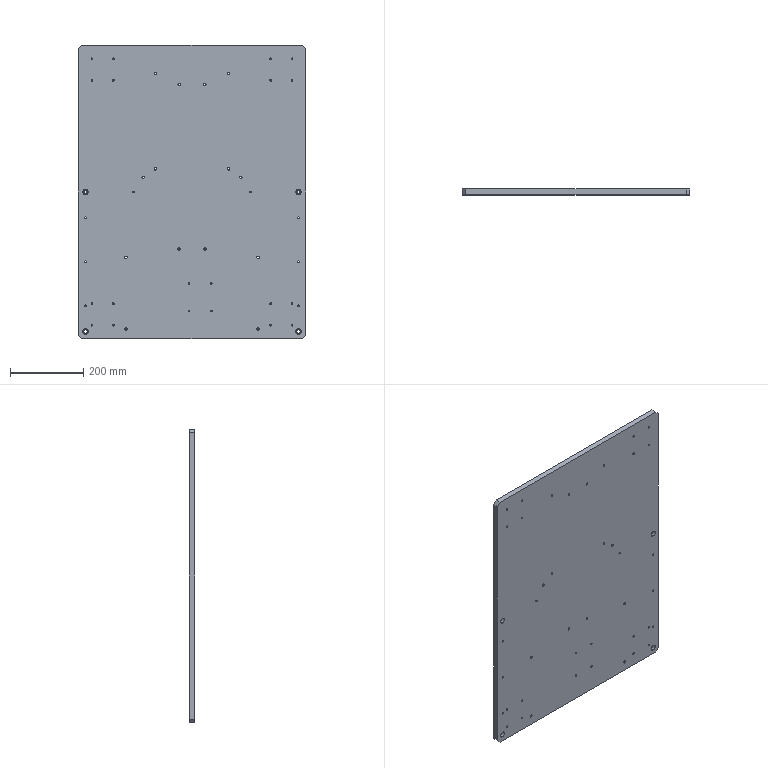Part | STEP file | PN_0010 | 1 solid | 138 faces | box 620 x 15 x 800 mm | volume 7409131 mm3 | cylinder 116 | plane 22 | commonest cylinder face diameters 5 x56 6.6 x24 20.2 x16 9 x8 15 x8 6.5 x4